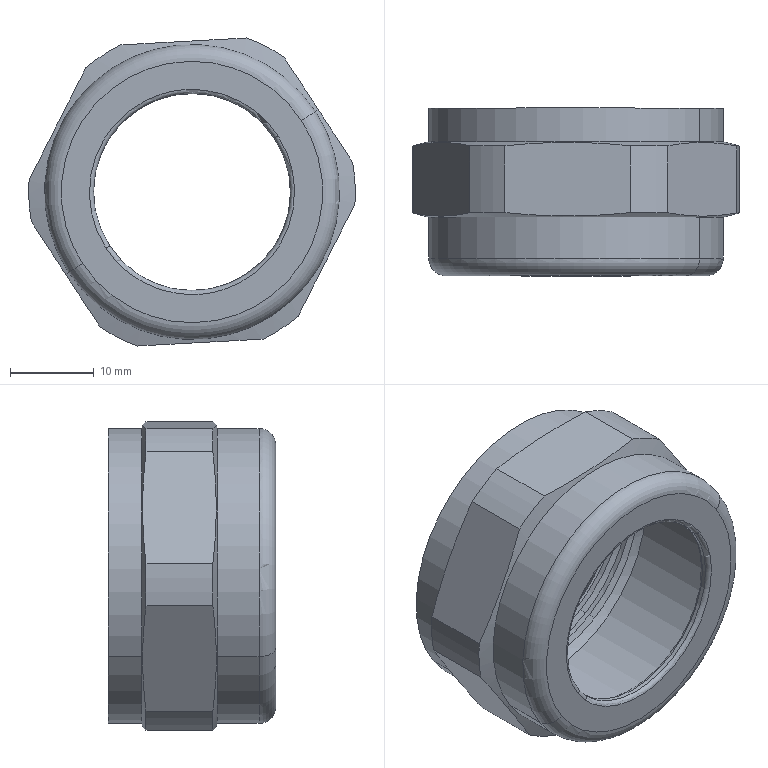Part | SolidWorks | features BaseBody 1 | 1 solid | 67 faces | box 39 x 20 x 36.772 mm | volume 4794 mm3 | spline 22 | cylinder 20 | plane 10 | cone 9 | torus 6 | commonest cylinder face diameters 30.6 x6 39 x6 35.2 x4 23.5 x2 32.5 x2